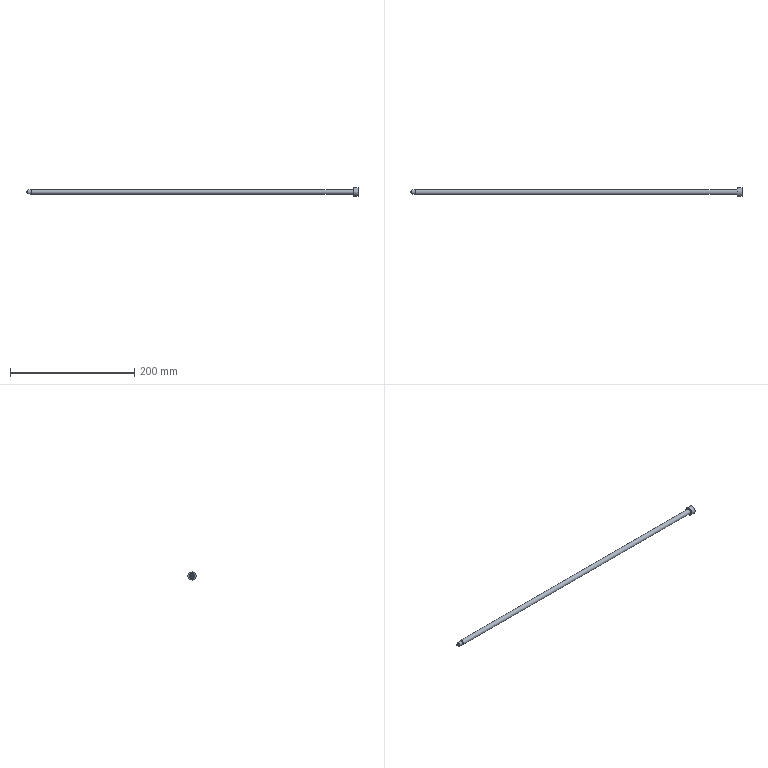Part | STEP file | solid 261 | 1 solid | 10 faces | box 533.706 x 13 x 13 mm | volume 27276 mm3 | plane 3 | cylinder 2 | spline 2 | cone 2 | torus 1 | commonest cylinder face diameters 8 x1 13 x1